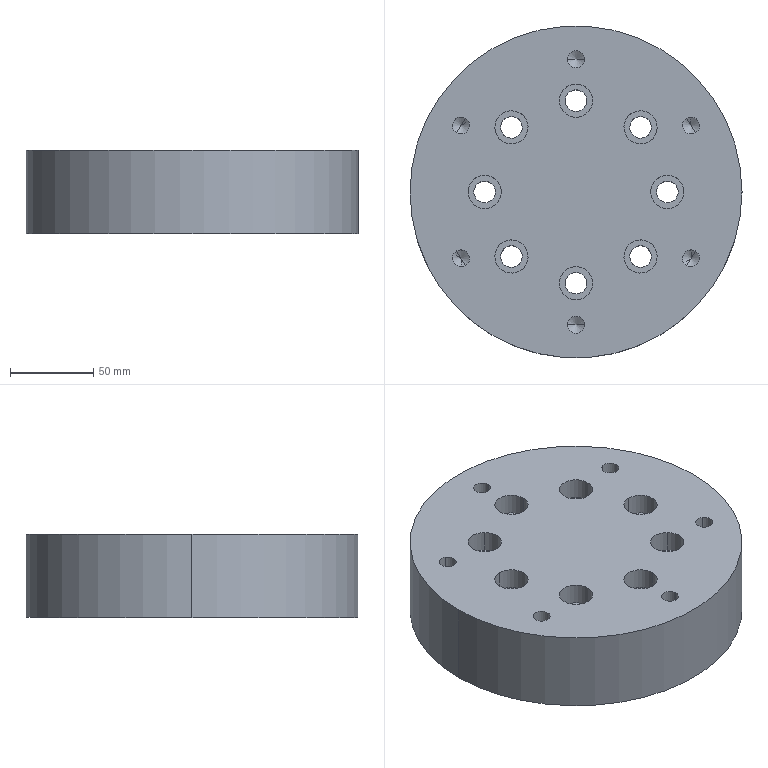Part | SolidWorks | features BaseBody 1 | 1 solid | 68 faces | box 200 x 200 x 50 mm | volume 1483994 mm3 | cylinder 46 | cone 12 | plane 10 | commonest cylinder face diameters 13 x16 20 x16 10.2 x12 200 x2